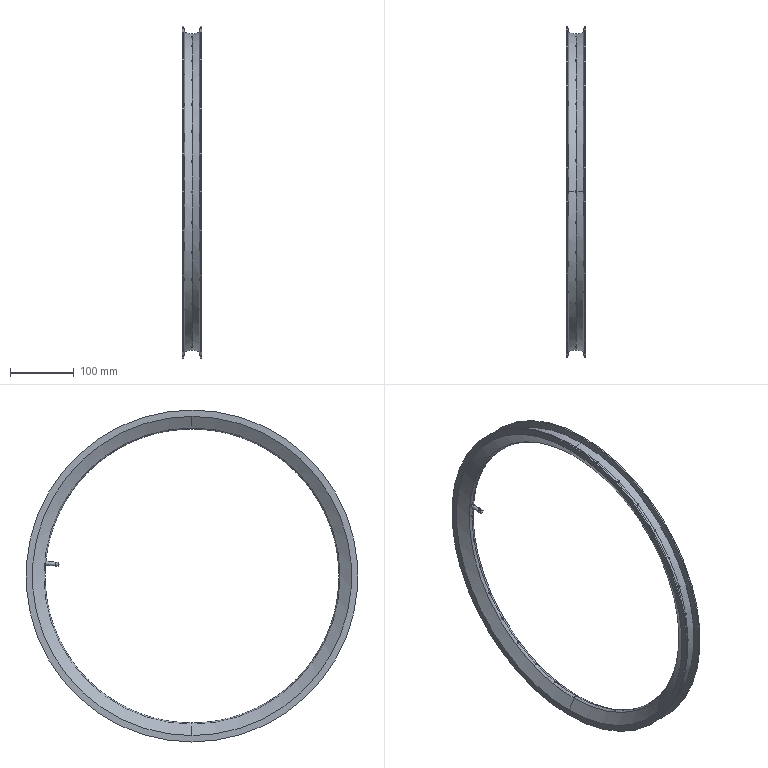Part | STEP file | Rear KMX Rim | 1 solid | 97 faces | box 30 x 520 x 520 mm | volume 578186 mm3 | cylinder 74 | cone 14 | plane 5 | torus 4 | commonest cylinder face diameters 3 x64 520 x4 4.755 x2 6 x2 6.4 x2